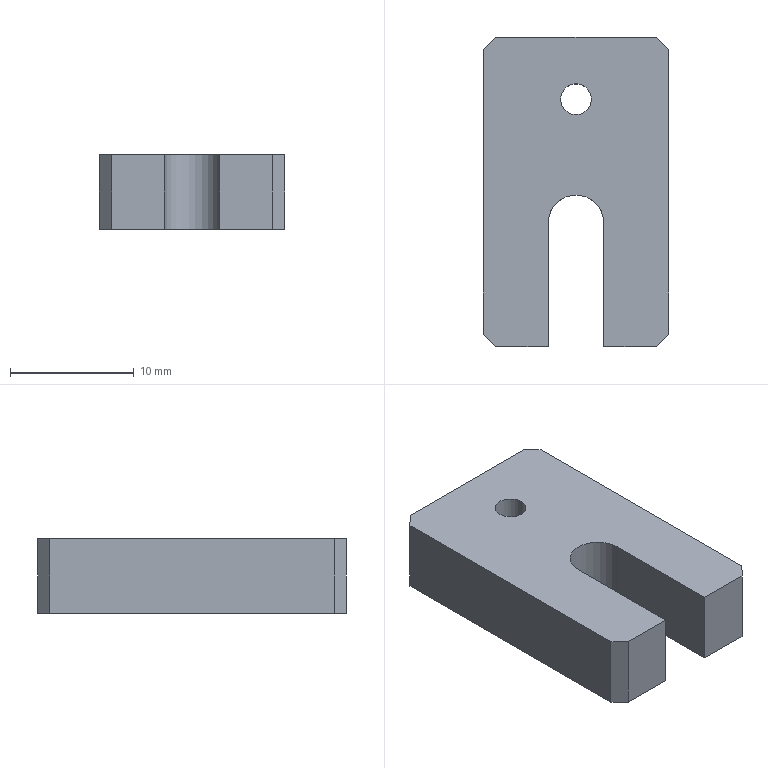Part | SolidWorks | features HoleWzd 2, Chamfer 1, Extrusion 1, ICE 1 | 1 solid | 16 faces | box 15 x 25 x 6 mm | volume 1891 mm3 | plane 13 | cylinder 3 | commonest cylinder face diameters 2.5 x2 4.5 x1
STEP:
#1=CARTESIAN_POINT('',(-1.25,10.,0.));
#2=VERTEX_POINT('',#1);
#3=CARTESIAN_POINT('',(1.25,10.,0.));
#4=VERTEX_POINT('',#3);
#5=CARTESIAN_POINT('',(0.,10.,0.));
#6=DIRECTION('',(0.,0.,1.));
#7=DIRECTION('',(1.,0.,0.));
#8=AXIS2_PLACEMENT_3D('',#5,#6,#7);
#9=CIRCLE('',#8,1.25);
#10=EDGE_CURVE('',#2,#4,#9,.T.);
#11=ORIENTED_EDGE('',*,*,#10,.F.);
#12=CARTESIAN_POINT('',(-1.25,10.,6.));
#13=VERTEX_POINT('',#12);
#14=CARTESIAN_POINT('',(-1.25,10.,6.));
#15=DIRECTION('',(0.,0.,1.));
#16=VECTOR('',#15,1000.);
#17=LINE('',#14,#16);
#18=EDGE_CURVE('',#2,#13,#17,.T.);
#19=ORIENTED_EDGE('',*,*,#18,.T.);
#20=CARTESIAN_POINT('',(1.25,10.,6.));
#21=VERTEX_POINT('',#20);
#22=CARTESIAN_POINT('',(0.,10.,6.));
#23=DIRECTION('',(0.,0.,1.));
#24=DIRECTION('',(1.,0.,0.));
#25=AXIS2_PLACEMENT_3D('',#22,#23,#24);
#26=CIRCLE('',#25,1.25);
#27=EDGE_CURVE('',#13,#21,#26,.T.);
#28=ORIENTED_EDGE('',*,*,#27,.T.);
#29=CARTESIAN_POINT('',(1.25,10.,6.));
#30=DIRECTION('',(0.,0.,1.));
#31=VECTOR('',#30,1000.);
#32=LINE('',#29,#31);
#33=EDGE_CURVE('',#4,#21,#32,.T.);
#34=ORIENTED_EDGE('',*,*,#33,.F.);
#35=EDGE_LOOP('',(#11,#19,#28,#34));
#36=FACE_OUTER_BOUND('',#35,.T.);
#37=CARTESIAN_POINT('',(0.,10.,6.));
#38=DIRECTION('',(0.,0.,1.));
#39=DIRECTION('',(1.,0.,0.));
#40=AXIS2_PLACEMENT_3D('',#37,#38,#39);
#41=CYLINDRICAL_SURFACE('',#40,1.25);
#42=ADVANCED_FACE('',(#36),#41,.F.);
#43=CARTESIAN_POINT('',(7.5,-9.,0.));
#44=VERTEX_POINT('',#43);
#45=CARTESIAN_POINT('',(7.5,14.,0.));
#46=VERTEX_POINT('',#45);
#47=CARTESIAN_POINT('',(7.5,15.,0.));
#48=DIRECTION('',(0.,1.,0.));
#49=VECTOR('',#48,1000.);
#50=LINE('',#47,#49);
#51=EDGE_CURVE('',#44,#46,#50,.T.);
#52=ORIENTED_EDGE('',*,*,#51,.T.);
#53=CARTESIAN_POINT('',(7.5,14.,6.));
#54=VERTEX_POINT('',#53);
#55=CARTESIAN_POINT('',(7.5,14.,6.));
#56=DIRECTION('',(0.,0.,1.));
#57=VECTOR('',#56,1000.);
#58=LINE('',#55,#57);
#59=EDGE_CURVE('',#46,#54,#58,.T.);
#60=ORIENTED_EDGE('',*,*,#59,.T.);
#61=CARTESIAN_POINT('',(7.5,-9.,6.));
#62=VERTEX_POINT('',#61);
#63=CARTESIAN_POINT('',(7.5,15.,6.));
#64=DIRECTION('',(0.,1.,0.));
#65=VECTOR('',#64,1000.);
#66=LINE('',#63,#65);
#67=EDGE_CURVE('',#62,#54,#66,.T.);
#68=ORIENTED_EDGE('',*,*,#67,.F.);
#69=CARTESIAN_POINT('',(7.5,-9.,6.));
#70=DIRECTION('',(0.,0.,-1.));
#71=VECTOR('',#70,1000.);
#72=LINE('',#69,#71);
#73=EDGE_CURVE('',#62,#44,#72,.T.);
#74=ORIENTED_EDGE('',*,*,#73,.T.);
#75=EDGE_LOOP('',(#52,#60,#68,#74));
#76=FACE_OUTER_BOUND('',#75,.T.);
#77=CARTESIAN_POINT('',(7.5,15.,6.));
#78=DIRECTION('',(-1.,0.,0.));
#79=DIRECTION('',(0.,-1.,0.));
#80=AXIS2_PLACEMENT_3D('',#77,#78,#79);
#81=PLANE('',#80);
#82=ADVANCED_FACE('',(#76),#81,.F.);
#83=CARTESIAN_POINT('',(6.5,15.,6.));
#84=VERTEX_POINT('',#83);
#85=CARTESIAN_POINT('',(-6.5,15.,6.));
#86=VERTEX_POINT('',#85);
#87=CARTESIAN_POINT('',(-7.5,15.,6.));
#88=DIRECTION('',(-1.,0.,0.));
#89=VECTOR('',#88,1000.);
#90=LINE('',#87,#89);
#91=EDGE_CURVE('',#84,#86,#90,.T.);
#92=ORIENTED_EDGE('',*,*,#91,.F.);
#93=CARTESIAN_POINT('',(6.5,15.,0.));
#94=VERTEX_POINT('',#93);
#95=CARTESIAN_POINT('',(6.5,15.,6.));
#96=DIRECTION('',(0.,0.,-1.));
#97=VECTOR('',#96,1000.);
#98=LINE('',#95,#97);
#99=EDGE_CURVE('',#84,#94,#98,.T.);
#100=ORIENTED_EDGE('',*,*,#99,.T.);
#101=CARTESIAN_POINT('',(-6.5,15.,0.));
#102=VERTEX_POINT('',#101);
#103=CARTESIAN_POINT('',(-7.5,15.,0.));
#104=DIRECTION('',(-1.,0.,0.));
#105=VECTOR('',#104,1000.);
#106=LINE('',#103,#105);
#107=EDGE_CURVE('',#94,#102,#106,.T.);
#108=ORIENTED_EDGE('',*,*,#107,.T.);
#109=CARTESIAN_POINT('',(-6.5,15.,6.));
#110=DIRECTION('',(0.,0.,1.));
#111=VECTOR('',#110,1000.);
#112=LINE('',#109,#111);
#113=EDGE_CURVE('',#102,#86,#112,.T.);
#114=ORIENTED_EDGE('',*,*,#113,.T.);
#115=EDGE_LOOP('',(#92,#100,#108,#114));
#116=FACE_OUTER_BOUND('',#115,.T.);
#117=CARTESIAN_POINT('',(-7.5,15.,6.));
#118=DIRECTION('',(0.,-1.,0.));
#119=DIRECTION('',(0.,0.,-1.));
#120=AXIS2_PLACEMENT_3D('',#117,#118,#119);
#121=PLANE('',#120);
#122=ADVANCED_FACE('',(#116),#121,.F.);
#123=CARTESIAN_POINT('',(-7.5,14.,6.));
#124=VERTEX_POINT('',#123);
#125=CARTESIAN_POINT('',(-7.5,-9.,6.));
#126=VERTEX_POINT('',#125);
#127=CARTESIAN_POINT('',(-7.5,15.,6.));
#128=DIRECTION('',(0.,-1.,0.));
#129=VECTOR('',#128,1000.);
#130=LINE('',#127,#129);
#131=EDGE_CURVE('',#124,#126,#130,.T.);
#132=ORIENTED_EDGE('',*,*,#131,.F.);
#133=CARTESIAN_POINT('',(-7.5,14.,0.));
#134=VERTEX_POINT('',#133);
#135=CARTESIAN_POINT('',(-7.5,14.,6.));
#136=DIRECTION('',(0.,0.,-1.));
#137=VECTOR('',#136,1000.);
#138=LINE('',#135,#137);
#139=EDGE_CURVE('',#124,#134,#138,.T.);
#140=ORIENTED_EDGE('',*,*,#139,.T.);
#141=CARTESIAN_POINT('',(-7.5,-9.,0.));
#142=VERTEX_POINT('',#141);
#143=CARTESIAN_POINT('',(-7.5,15.,0.));
#144=DIRECTION('',(0.,-1.,0.));
#145=VECTOR('',#144,1000.);
#146=LINE('',#143,#145);
#147=EDGE_CURVE('',#134,#142,#146,.T.);
#148=ORIENTED_EDGE('',*,*,#147,.T.);
#149=CARTESIAN_POINT('',(-7.5,-9.,6.));
#150=DIRECTION('',(0.,0.,1.));
#151=VECTOR('',#150,1000.);
#152=LINE('',#149,#151);
#153=EDGE_CURVE('',#142,#126,#152,.T.);
#154=ORIENTED_EDGE('',*,*,#153,.T.);
#155=EDGE_LOOP('',(#132,#140,#148,#154));
#156=FACE_OUTER_BOUND('',#155,.T.);
#157=CARTESIAN_POINT('',(-7.5,15.,6.));
#158=DIRECTION('',(1.,0.,0.));
#159=DIRECTION('',(0.,1.,0.));
#160=AXIS2_PLACEMENT_3D('',#157,#158,#159);
#161=PLANE('',#160);
#162=ADVANCED_FACE('',(#156),#161,.F.);
#163=ORIENTED_EDGE('',*,*,#67,.T.);
#164=CARTESIAN_POINT('',(10.75,10.75,6.));
#165=DIRECTION('',(-0.7071,0.7071,0.));
#166=VECTOR('',#165,1000.);
#167=LINE('',#164,#166);
#168=EDGE_CURVE('',#54,#84,#167,.T.);
#169=ORIENTED_EDGE('',*,*,#168,.T.);
#170=ORIENTED_EDGE('',*,*,#91,.T.);
#171=CARTESIAN_POINT('',(-10.75,10.75,6.));
#172=DIRECTION('',(-0.7071,-0.7071,0.));
#173=VECTOR('',#172,1000.);
#174=LINE('',#171,#173);
#175=EDGE_CURVE('',#86,#124,#174,.T.);
#176=ORIENTED_EDGE('',*,*,#175,.T.);
#177=ORIENTED_EDGE('',*,*,#131,.T.);
#178=CARTESIAN_POINT('',(-6.5,-10.,6.));
#179=VERTEX_POINT('',#178);
#180=CARTESIAN_POINT('',(-8.25,-8.25,6.));
#181=DIRECTION('',(0.7071,-0.7071,0.));
#182=VECTOR('',#181,1000.);
#183=LINE('',#180,#182);
#184=EDGE_CURVE('',#126,#179,#183,.T.);
#185=ORIENTED_EDGE('',*,*,#184,.T.);
#186=CARTESIAN_POINT('',(-2.25,-10.,6.));
#187=VERTEX_POINT('',#186);
#188=CARTESIAN_POINT('',(-7.5,-10.,6.));
#189=DIRECTION('',(-1.,0.,0.));
#190=VECTOR('',#189,1000.);
#191=LINE('',#188,#190);
#192=EDGE_CURVE('',#187,#179,#191,.T.);
#193=ORIENTED_EDGE('',*,*,#192,.F.);
#194=CARTESIAN_POINT('',(-2.25,0.,6.));
#195=VERTEX_POINT('',#194);
#196=CARTESIAN_POINT('',(-2.25,0.,6.));
#197=DIRECTION('',(0.,-1.,0.));
#198=VECTOR('',#197,1000.);
#199=LINE('',#196,#198);
#200=EDGE_CURVE('',#195,#187,#199,.T.);
#201=ORIENTED_EDGE('',*,*,#200,.F.);
#202=CARTESIAN_POINT('',(2.25,0.,6.));
#203=VERTEX_POINT('',#202);
#204=CARTESIAN_POINT('',(0.,0.,6.));
#205=DIRECTION('',(0.,0.,1.));
#206=DIRECTION('',(1.,0.,0.));
#207=AXIS2_PLACEMENT_3D('',#204,#205,#206);
#208=CIRCLE('',#207,2.25);
#209=EDGE_CURVE('',#203,#195,#208,.T.);
#210=ORIENTED_EDGE('',*,*,#209,.F.);
#211=CARTESIAN_POINT('',(2.25,-10.,6.));
#212=VERTEX_POINT('',#211);
#213=CARTESIAN_POINT('',(2.25,0.,6.));
#214=DIRECTION('',(0.,-1.,0.));
#215=VECTOR('',#214,1000.);
#216=LINE('',#213,#215);
#217=EDGE_CURVE('',#203,#212,#216,.T.);
#218=ORIENTED_EDGE('',*,*,#217,.T.);
#219=CARTESIAN_POINT('',(6.5,-10.,6.));
#220=VERTEX_POINT('',#219);
#221=CARTESIAN_POINT('',(-7.5,-10.,6.));
#222=DIRECTION('',(-1.,0.,0.));
#223=VECTOR('',#222,1000.);
#224=LINE('',#221,#223);
#225=EDGE_CURVE('',#220,#212,#224,.T.);
#226=ORIENTED_EDGE('',*,*,#225,.F.);
#227=CARTESIAN_POINT('',(8.25,-8.25,6.));
#228=DIRECTION('',(0.7071,0.7071,0.));
#229=VECTOR('',#228,1000.);
#230=LINE('',#227,#229);
#231=EDGE_CURVE('',#220,#62,#230,.T.);
#232=ORIENTED_EDGE('',*,*,#231,.T.);
#233=EDGE_LOOP('',(#163,#169,#170,#176,#177,#185,#193,#201,#210,#218,#226,#232));
#234=FACE_OUTER_BOUND('',#233,.T.);
#235=CARTESIAN_POINT('',(0.,10.,6.));
#236=DIRECTION('',(0.,0.,1.));
#237=DIRECTION('',(1.,0.,0.));
#238=AXIS2_PLACEMENT_3D('',#235,#236,#237);
#239=CIRCLE('',#238,1.25);
#240=EDGE_CURVE('',#21,#13,#239,.T.);
#241=ORIENTED_EDGE('',*,*,#240,.F.);
#242=ORIENTED_EDGE('',*,*,#27,.F.);
#243=EDGE_LOOP('',(#241,#242));
#244=FACE_BOUND('',#243,.T.);
#245=CARTESIAN_POINT('',(0.,0.,6.));
#246=DIRECTION('',(0.,0.,1.));
#247=DIRECTION('',(1.,0.,0.));
#248=AXIS2_PLACEMENT_3D('',#245,#246,#247);
#249=PLANE('',#248);
#250=ADVANCED_FACE('',(#234,#244),#249,.T.);
#251=ORIENTED_EDGE('',*,*,#107,.F.);
#252=CARTESIAN_POINT('',(6.5,15.,0.));
#253=DIRECTION('',(0.7071,-0.7071,0.));
#254=VECTOR('',#253,1000.);
#255=LINE('',#252,#254);
#256=EDGE_CURVE('',#94,#46,#255,.T.);
#257=ORIENTED_EDGE('',*,*,#256,.T.);
#258=ORIENTED_EDGE('',*,*,#51,.F.);
#259=CARTESIAN_POINT('',(6.5,-10.,0.));
#260=VERTEX_POINT('',#259);
#261=CARTESIAN_POINT('',(6.5,-10.,0.));
#262=DIRECTION('',(-0.7071,-0.7071,0.));
#263=VECTOR('',#262,1000.);
#264=LINE('',#261,#263);
#265=EDGE_CURVE('',#44,#260,#264,.T.);
#266=ORIENTED_EDGE('',*,*,#265,.T.);
#267=CARTESIAN_POINT('',(2.25,-10.,0.));
#268=VERTEX_POINT('',#267);
#269=CARTESIAN_POINT('',(-7.5,-10.,0.));
#270=DIRECTION('',(-1.,0.,0.));
#271=VECTOR('',#270,1000.);
#272=LINE('',#269,#271);
#273=EDGE_CURVE('',#260,#268,#272,.T.);
#274=ORIENTED_EDGE('',*,*,#273,.T.);
#275=CARTESIAN_POINT('',(2.25,0.,0.));
#276=VERTEX_POINT('',#275);
#277=CARTESIAN_POINT('',(2.25,0.,0.));
#278=DIRECTION('',(0.,-1.,0.));
#279=VECTOR('',#278,1000.);
#280=LINE('',#277,#279);
#281=EDGE_CURVE('',#276,#268,#280,.T.);
#282=ORIENTED_EDGE('',*,*,#281,.F.);
#283=CARTESIAN_POINT('',(-2.25,0.,0.));
#284=VERTEX_POINT('',#283);
#285=CARTESIAN_POINT('',(0.,0.,0.));
#286=DIRECTION('',(0.,0.,1.));
#287=DIRECTION('',(1.,0.,0.));
#288=AXIS2_PLACEMENT_3D('',#285,#286,#287);
#289=CIRCLE('',#288,2.25);
#290=EDGE_CURVE('',#276,#284,#289,.T.);
#291=ORIENTED_EDGE('',*,*,#290,.T.);
#292=CARTESIAN_POINT('',(-2.25,-10.,0.));
#293=VERTEX_POINT('',#292);
#294=CARTESIAN_POINT('',(-2.25,0.,0.));
#295=DIRECTION('',(0.,-1.,0.));
#296=VECTOR('',#295,1000.);
#297=LINE('',#294,#296);
#298=EDGE_CURVE('',#284,#293,#297,.T.);
#299=ORIENTED_EDGE('',*,*,#298,.T.);
#300=CARTESIAN_POINT('',(-6.5,-10.,0.));
#301=VERTEX_POINT('',#300);
#302=CARTESIAN_POINT('',(-7.5,-10.,0.));
#303=DIRECTION('',(-1.,0.,0.));
#304=VECTOR('',#303,1000.);
#305=LINE('',#302,#304);
#306=EDGE_CURVE('',#293,#301,#305,.T.);
#307=ORIENTED_EDGE('',*,*,#306,.T.);
#308=CARTESIAN_POINT('',(-7.5,-9.,0.));
#309=DIRECTION('',(-0.7071,0.7071,0.));
#310=VECTOR('',#309,1000.);
#311=LINE('',#308,#310);
#312=EDGE_CURVE('',#301,#142,#311,.T.);
#313=ORIENTED_EDGE('',*,*,#312,.T.);
#314=ORIENTED_EDGE('',*,*,#147,.F.);
#315=CARTESIAN_POINT('',(-7.5,14.,0.));
#316=DIRECTION('',(0.7071,0.7071,0.));
#317=VECTOR('',#316,1000.);
#318=LINE('',#315,#317);
#319=EDGE_CURVE('',#134,#102,#318,.T.);
#320=ORIENTED_EDGE('',*,*,#319,.T.);
#321=EDGE_LOOP('',(#251,#257,#258,#266,#274,#282,#291,#299,#307,#313,#314,#320));
#322=FACE_OUTER_BOUND('',#321,.T.);
#323=CARTESIAN_POINT('',(0.,10.,0.));
#324=DIRECTION('',(0.,0.,1.));
#325=DIRECTION('',(1.,0.,0.));
#326=AXIS2_PLACEMENT_3D('',#323,#324,#325);
#327=CIRCLE('',#326,1.25);
#328=EDGE_CURVE('',#4,#2,#327,.T.);
#329=ORIENTED_EDGE('',*,*,#328,.T.);
#330=ORIENTED_EDGE('',*,*,#10,.T.);
#331=EDGE_LOOP('',(#329,#330));
#332=FACE_BOUND('',#331,.T.);
#333=CARTESIAN_POINT('',(0.,0.,0.));
#334=DIRECTION('',(0.,0.,1.));
#335=DIRECTION('',(1.,0.,0.));
#336=AXIS2_PLACEMENT_3D('',#333,#334,#335);
#337=PLANE('',#336);
#338=ADVANCED_FACE('',(#322,#332),#337,.F.);
#339=ORIENTED_EDGE('',*,*,#18,.F.);
#340=ORIENTED_EDGE('',*,*,#328,.F.);
#341=ORIENTED_EDGE('',*,*,#33,.T.);
#342=ORIENTED_EDGE('',*,*,#240,.T.);
#343=EDGE_LOOP('',(#339,#340,#341,#342));
#344=FACE_OUTER_BOUND('',#343,.T.);
#345=CARTESIAN_POINT('',(0.,10.,6.));
#346=DIRECTION('',(0.,0.,1.));
#347=DIRECTION('',(1.,0.,0.));
#348=AXIS2_PLACEMENT_3D('',#345,#346,#347);
#349=CYLINDRICAL_SURFACE('',#348,1.25);
#350=ADVANCED_FACE('',(#344),#349,.F.);
#351=ORIENTED_EDGE('',*,*,#290,.F.);
#352=CARTESIAN_POINT('',(2.25,0.,0.));
#353=DIRECTION('',(0.,0.,-1.));
#354=VECTOR('',#353,1000.);
#355=LINE('',#352,#354);
#356=EDGE_CURVE('',#203,#276,#355,.T.);
#357=ORIENTED_EDGE('',*,*,#356,.F.);
#358=ORIENTED_EDGE('',*,*,#209,.T.);
#359=CARTESIAN_POINT('',(-2.25,0.,6.));
#360=DIRECTION('',(0.,0.,1.));
#361=VECTOR('',#360,1000.);
#362=LINE('',#359,#361);
#363=EDGE_CURVE('',#284,#195,#362,.T.);
#364=ORIENTED_EDGE('',*,*,#363,.F.);
#365=EDGE_LOOP('',(#351,#357,#358,#364));
#366=FACE_OUTER_BOUND('',#365,.T.);
#367=CARTESIAN_POINT('',(0.,0.,6.));
#368=DIRECTION('',(0.,0.,1.));
#369=DIRECTION('',(1.,0.,0.));
#370=AXIS2_PLACEMENT_3D('',#367,#368,#369);
#371=CYLINDRICAL_SURFACE('',#370,2.25);
#372=ADVANCED_FACE('',(#366),#371,.F.);
#373=CARTESIAN_POINT('',(2.25,-10.,0.));
#374=DIRECTION('',(0.,0.,-1.));
#375=VECTOR('',#374,1000.);
#376=LINE('',#373,#375);
#377=EDGE_CURVE('',#212,#268,#376,.T.);
#378=ORIENTED_EDGE('',*,*,#377,.F.);
#379=ORIENTED_EDGE('',*,*,#217,.F.);
#380=ORIENTED_EDGE('',*,*,#356,.T.);
#381=ORIENTED_EDGE('',*,*,#281,.T.);
#382=EDGE_LOOP('',(#378,#379,#380,#381));
#383=FACE_OUTER_BOUND('',#382,.T.);
#384=CARTESIAN_POINT('',(2.25,0.,0.));
#385=DIRECTION('',(-1.,0.,0.));
#386=DIRECTION('',(0.,-1.,0.));
#387=AXIS2_PLACEMENT_3D('',#384,#385,#386);
#388=PLANE('',#387);
#389=ADVANCED_FACE('',(#383),#388,.T.);
#390=CARTESIAN_POINT('',(-2.25,-10.,6.));
#391=DIRECTION('',(0.,0.,-1.));
#392=VECTOR('',#391,1000.);
#393=LINE('',#390,#392);
#394=EDGE_CURVE('',#187,#293,#393,.T.);
#395=ORIENTED_EDGE('',*,*,#394,.T.);
#396=ORIENTED_EDGE('',*,*,#298,.F.);
#397=ORIENTED_EDGE('',*,*,#363,.T.);
#398=ORIENTED_EDGE('',*,*,#200,.T.);
#399=EDGE_LOOP('',(#395,#396,#397,#398));
#400=FACE_OUTER_BOUND('',#399,.T.);
#401=CARTESIAN_POINT('',(-2.25,0.,6.));
#402=DIRECTION('',(-1.,0.,0.));
#403=DIRECTION('',(0.,-1.,0.));
#404=AXIS2_PLACEMENT_3D('',#401,#402,#403);
#405=PLANE('',#404);
#406=ADVANCED_FACE('',(#400),#405,.F.);
#407=ORIENTED_EDGE('',*,*,#192,.T.);
#408=CARTESIAN_POINT('',(-6.5,-10.,0.));
#409=DIRECTION('',(0.,0.,-1.));
#410=VECTOR('',#409,1000.);
#411=LINE('',#408,#410);
#412=EDGE_CURVE('',#179,#301,#411,.T.);
#413=ORIENTED_EDGE('',*,*,#412,.T.);
#414=ORIENTED_EDGE('',*,*,#306,.F.);
#415=ORIENTED_EDGE('',*,*,#394,.F.);
#416=EDGE_LOOP('',(#407,#413,#414,#415));
#417=FACE_OUTER_BOUND('',#416,.T.);
#418=CARTESIAN_POINT('',(-7.5,-10.,0.));
#419=DIRECTION('',(0.,1.,0.));
#420=DIRECTION('',(0.,0.,1.));
#421=AXIS2_PLACEMENT_3D('',#418,#419,#420);
#422=PLANE('',#421);
#423=ADVANCED_FACE('',(#417),#422,.F.);
#424=ORIENTED_EDGE('',*,*,#273,.F.);
#425=CARTESIAN_POINT('',(6.5,-10.,0.));
#426=DIRECTION('',(0.,0.,1.));
#427=VECTOR('',#426,1000.);
#428=LINE('',#425,#427);
#429=EDGE_CURVE('',#260,#220,#428,.T.);
#430=ORIENTED_EDGE('',*,*,#429,.T.);
#431=ORIENTED_EDGE('',*,*,#225,.T.);
#432=ORIENTED_EDGE('',*,*,#377,.T.);
#433=EDGE_LOOP('',(#424,#430,#431,#432));
#434=FACE_OUTER_BOUND('',#433,.T.);
#435=CARTESIAN_POINT('',(-7.5,-10.,0.));
#436=DIRECTION('',(0.,1.,0.));
#437=DIRECTION('',(0.,0.,1.));
#438=AXIS2_PLACEMENT_3D('',#435,#436,#437);
#439=PLANE('',#438);
#440=ADVANCED_FACE('',(#434),#439,.F.);
#441=ORIENTED_EDGE('',*,*,#168,.F.);
#442=ORIENTED_EDGE('',*,*,#59,.F.);
#443=ORIENTED_EDGE('',*,*,#256,.F.);
#444=ORIENTED_EDGE('',*,*,#99,.F.);
#445=EDGE_LOOP('',(#441,#442,#443,#444));
#446=FACE_OUTER_BOUND('',#445,.T.);
#447=CARTESIAN_POINT('',(6.5,15.,6.));
#448=DIRECTION('',(-0.7071,-0.7071,0.));
#449=DIRECTION('',(0.,0.,-1.));
#450=AXIS2_PLACEMENT_3D('',#447,#448,#449);
#451=PLANE('',#450);
#452=ADVANCED_FACE('',(#446),#451,.F.);
#453=ORIENTED_EDGE('',*,*,#175,.F.);
#454=ORIENTED_EDGE('',*,*,#113,.F.);
#455=ORIENTED_EDGE('',*,*,#319,.F.);
#456=ORIENTED_EDGE('',*,*,#139,.F.);
#457=EDGE_LOOP('',(#453,#454,#455,#456));
#458=FACE_OUTER_BOUND('',#457,.T.);
#459=CARTESIAN_POINT('',(-7.5,14.,6.));
#460=DIRECTION('',(0.7071,-0.7071,0.));
#461=DIRECTION('',(0.,0.,-1.));
#462=AXIS2_PLACEMENT_3D('',#459,#460,#461);
#463=PLANE('',#462);
#464=ADVANCED_FACE('',(#458),#463,.F.);
#465=ORIENTED_EDGE('',*,*,#265,.F.);
#466=ORIENTED_EDGE('',*,*,#73,.F.);
#467=ORIENTED_EDGE('',*,*,#231,.F.);
#468=ORIENTED_EDGE('',*,*,#429,.F.);
#469=EDGE_LOOP('',(#465,#466,#467,#468));
#470=FACE_OUTER_BOUND('',#469,.T.);
#471=CARTESIAN_POINT('',(6.5,-10.,0.));
#472=DIRECTION('',(-0.7071,0.7071,0.));
#473=DIRECTION('',(0.,0.,1.));
#474=AXIS2_PLACEMENT_3D('',#471,#472,#473);
#475=PLANE('',#474);
#476=ADVANCED_FACE('',(#470),#475,.F.);
#477=ORIENTED_EDGE('',*,*,#312,.F.);
#478=ORIENTED_EDGE('',*,*,#412,.F.);
#479=ORIENTED_EDGE('',*,*,#184,.F.);
#480=ORIENTED_EDGE('',*,*,#153,.F.);
#481=EDGE_LOOP('',(#477,#478,#479,#480));
#482=FACE_OUTER_BOUND('',#481,.T.);
#483=CARTESIAN_POINT('',(-7.5,-9.,6.));
#484=DIRECTION('',(0.7071,0.7071,0.));
#485=DIRECTION('',(0.,0.,1.));
#486=AXIS2_PLACEMENT_3D('',#483,#484,#485);
#487=PLANE('',#486);
#488=ADVANCED_FACE('',(#482),#487,.F.);
#489=CLOSED_SHELL('',(#42,#82,#122,#162,#250,#338,#350,#372,#389,#406,#423,#440,#452,#464,#476,#488));
#490=MANIFOLD_SOLID_BREP('',#489);
#491=CARTESIAN_POINT('',(0.,0.,0.));
#492=DIRECTION('',(0.,0.,1.));
#493=DIRECTION('',(1.,0.,0.));
#494=AXIS2_PLACEMENT_3D('',#491,#492,#493);
#495=(LENGTH_UNIT()NAMED_UNIT(*)SI_UNIT(.MILLI.,.METRE.));
#496=UNCERTAINTY_MEASURE_WITH_UNIT(LENGTH_MEASURE(0.00001),#495,'','');
#497=(NAMED_UNIT(*)PLANE_ANGLE_UNIT()SI_UNIT($,.RADIAN.));
#498=(NAMED_UNIT(*)SI_UNIT($,.STERADIAN.)SOLID_ANGLE_UNIT());
#499=(GEOMETRIC_REPRESENTATION_CONTEXT(3)GLOBAL_UNCERTAINTY_ASSIGNED_CONTEXT((#496))GLOBAL_UNIT_ASSIGNED_CONTEXT((#495,#497,#498))REPRESENTATION_CONTEXT('',''));
#500=ADVANCED_BREP_SHAPE_REPRESENTATION('',(#490,#494),#499);